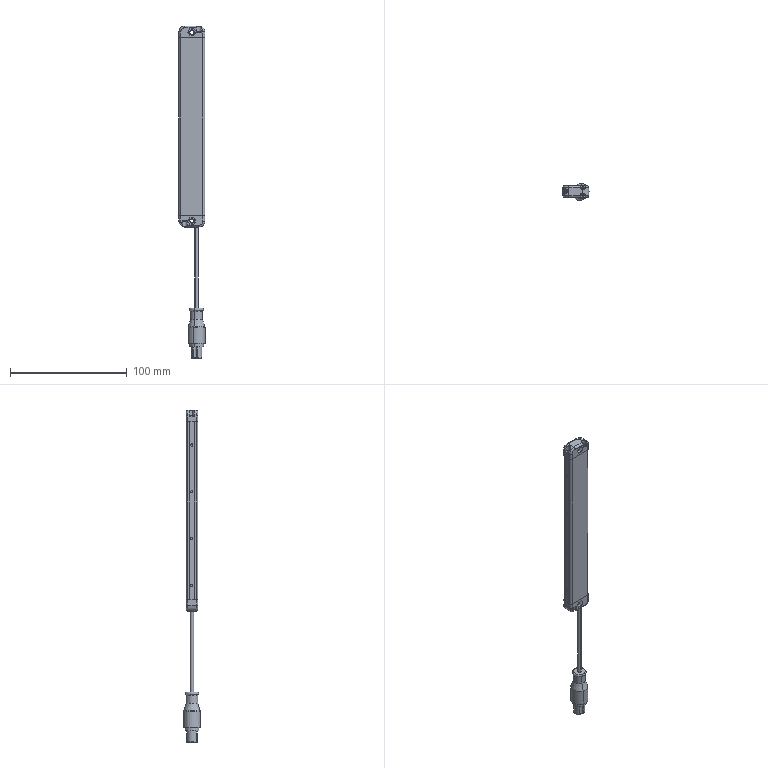Part | STEP file | Safety light curtain 4PLN-0440-P V1.201001 | 5 solids | 596 faces | box 22.25 x 14.5 x 284 mm | volume 22094 mm3 | cylinder 258 | plane 208 | torus 100 | spline 28 | cone 2 | commonest cylinder face diameters 0.4 x93 0.2 x26 3 x20 3.9 x16 0.6 x15 1.5 x12